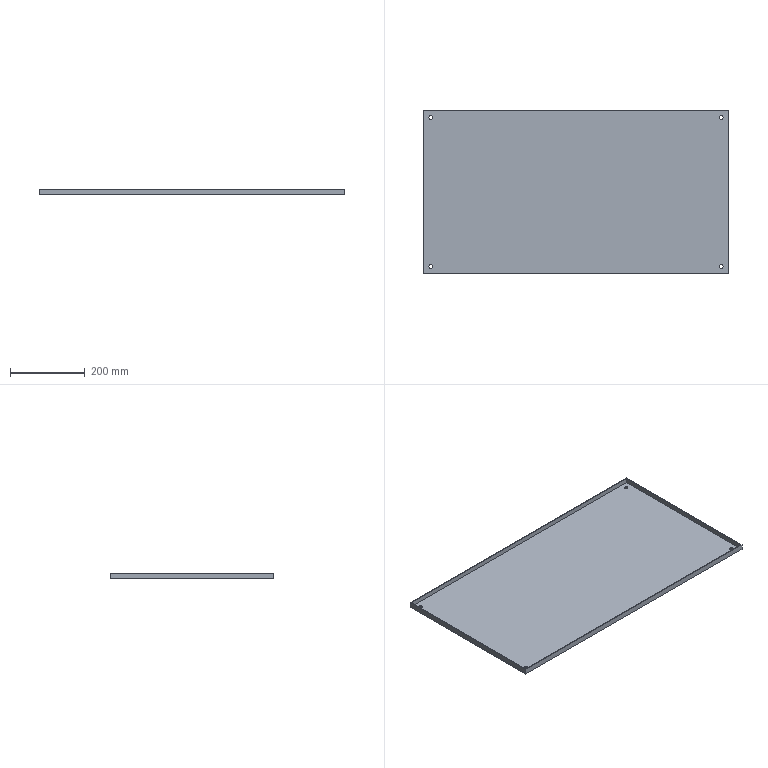Part | STEP file | 11-FGJJ-01111 | 1 solid | 19 faces | box 820 x 440 x 15 mm | volume 786284 mm3 | plane 11 | cylinder 8 | commonest cylinder face diameters 10 x8
STEP:
#1=CARTESIAN_POINT('',(-395.,200.,2.));
#2=VERTEX_POINT('',#1);
#3=CARTESIAN_POINT('',(-385.,200.,2.));
#4=VERTEX_POINT('',#3);
#5=CARTESIAN_POINT('',(-390.,200.,2.));
#6=DIRECTION('',(0.,0.,1.));
#7=DIRECTION('',(1.,0.,0.));
#8=AXIS2_PLACEMENT_3D('',#5,#6,#7);
#9=CIRCLE('',#8,5.);
#10=EDGE_CURVE('',#2,#4,#9,.T.);
#11=ORIENTED_EDGE('',*,*,#10,.T.);
#12=CARTESIAN_POINT('',(-385.,200.,0.));
#13=VERTEX_POINT('',#12);
#14=CARTESIAN_POINT('',(-385.,200.,44.));
#15=DIRECTION('',(0.,0.,-1.));
#16=VECTOR('',#15,1000.);
#17=LINE('',#14,#16);
#18=EDGE_CURVE('',#4,#13,#17,.T.);
#19=ORIENTED_EDGE('',*,*,#18,.T.);
#20=CARTESIAN_POINT('',(-395.,200.,0.));
#21=VERTEX_POINT('',#20);
#22=CARTESIAN_POINT('',(-390.,200.,0.));
#23=DIRECTION('',(0.,0.,-1.));
#24=DIRECTION('',(-1.,0.,0.));
#25=AXIS2_PLACEMENT_3D('',#22,#23,#24);
#26=CIRCLE('',#25,5.);
#27=EDGE_CURVE('',#13,#21,#26,.T.);
#28=ORIENTED_EDGE('',*,*,#27,.T.);
#29=CARTESIAN_POINT('',(-395.,200.,44.));
#30=DIRECTION('',(0.,0.,-1.));
#31=VECTOR('',#30,1000.);
#32=LINE('',#29,#31);
#33=EDGE_CURVE('',#2,#21,#32,.T.);
#34=ORIENTED_EDGE('',*,*,#33,.F.);
#35=EDGE_LOOP('',(#11,#19,#28,#34));
#36=FACE_OUTER_BOUND('',#35,.T.);
#37=CARTESIAN_POINT('',(-390.,200.,44.));
#38=DIRECTION('',(0.,0.,-1.));
#39=DIRECTION('',(-1.,0.,0.));
#40=AXIS2_PLACEMENT_3D('',#37,#38,#39);
#41=CYLINDRICAL_SURFACE('',#40,5.);
#42=ADVANCED_FACE('',(#36),#41,.F.);
#43=CARTESIAN_POINT('',(385.,-200.,2.));
#44=VERTEX_POINT('',#43);
#45=CARTESIAN_POINT('',(395.,-200.,2.));
#46=VERTEX_POINT('',#45);
#47=CARTESIAN_POINT('',(390.,-200.,2.));
#48=DIRECTION('',(0.,0.,1.));
#49=DIRECTION('',(1.,0.,0.));
#50=AXIS2_PLACEMENT_3D('',#47,#48,#49);
#51=CIRCLE('',#50,5.);
#52=EDGE_CURVE('',#44,#46,#51,.T.);
#53=ORIENTED_EDGE('',*,*,#52,.T.);
#54=CARTESIAN_POINT('',(395.,-200.,0.));
#55=VERTEX_POINT('',#54);
#56=CARTESIAN_POINT('',(395.,-200.,44.));
#57=DIRECTION('',(0.,0.,-1.));
#58=VECTOR('',#57,1000.);
#59=LINE('',#56,#58);
#60=EDGE_CURVE('',#46,#55,#59,.T.);
#61=ORIENTED_EDGE('',*,*,#60,.T.);
#62=CARTESIAN_POINT('',(385.,-200.,0.));
#63=VERTEX_POINT('',#62);
#64=CARTESIAN_POINT('',(390.,-200.,0.));
#65=DIRECTION('',(0.,0.,-1.));
#66=DIRECTION('',(-1.,0.,0.));
#67=AXIS2_PLACEMENT_3D('',#64,#65,#66);
#68=CIRCLE('',#67,5.);
#69=EDGE_CURVE('',#55,#63,#68,.T.);
#70=ORIENTED_EDGE('',*,*,#69,.T.);
#71=CARTESIAN_POINT('',(385.,-200.,44.));
#72=DIRECTION('',(0.,0.,-1.));
#73=VECTOR('',#72,1000.);
#74=LINE('',#71,#73);
#75=EDGE_CURVE('',#44,#63,#74,.T.);
#76=ORIENTED_EDGE('',*,*,#75,.F.);
#77=EDGE_LOOP('',(#53,#61,#70,#76));
#78=FACE_OUTER_BOUND('',#77,.T.);
#79=CARTESIAN_POINT('',(390.,-200.,44.));
#80=DIRECTION('',(0.,0.,-1.));
#81=DIRECTION('',(-1.,0.,0.));
#82=AXIS2_PLACEMENT_3D('',#79,#80,#81);
#83=CYLINDRICAL_SURFACE('',#82,5.);
#84=ADVANCED_FACE('',(#78),#83,.F.);
#85=CARTESIAN_POINT('',(-395.,-200.,2.));
#86=VERTEX_POINT('',#85);
#87=CARTESIAN_POINT('',(-385.,-200.,2.));
#88=VERTEX_POINT('',#87);
#89=CARTESIAN_POINT('',(-390.,-200.,2.));
#90=DIRECTION('',(0.,0.,1.));
#91=DIRECTION('',(1.,0.,0.));
#92=AXIS2_PLACEMENT_3D('',#89,#90,#91);
#93=CIRCLE('',#92,5.);
#94=EDGE_CURVE('',#86,#88,#93,.T.);
#95=ORIENTED_EDGE('',*,*,#94,.T.);
#96=CARTESIAN_POINT('',(-385.,-200.,0.));
#97=VERTEX_POINT('',#96);
#98=CARTESIAN_POINT('',(-385.,-200.,44.));
#99=DIRECTION('',(0.,0.,-1.));
#100=VECTOR('',#99,1000.);
#101=LINE('',#98,#100);
#102=EDGE_CURVE('',#88,#97,#101,.T.);
#103=ORIENTED_EDGE('',*,*,#102,.T.);
#104=CARTESIAN_POINT('',(-395.,-200.,0.));
#105=VERTEX_POINT('',#104);
#106=CARTESIAN_POINT('',(-390.,-200.,0.));
#107=DIRECTION('',(0.,0.,-1.));
#108=DIRECTION('',(-1.,0.,0.));
#109=AXIS2_PLACEMENT_3D('',#106,#107,#108);
#110=CIRCLE('',#109,5.);
#111=EDGE_CURVE('',#97,#105,#110,.T.);
#112=ORIENTED_EDGE('',*,*,#111,.T.);
#113=CARTESIAN_POINT('',(-395.,-200.,44.));
#114=DIRECTION('',(0.,0.,-1.));
#115=VECTOR('',#114,1000.);
#116=LINE('',#113,#115);
#117=EDGE_CURVE('',#86,#105,#116,.T.);
#118=ORIENTED_EDGE('',*,*,#117,.F.);
#119=EDGE_LOOP('',(#95,#103,#112,#118));
#120=FACE_OUTER_BOUND('',#119,.T.);
#121=CARTESIAN_POINT('',(-390.,-200.,44.));
#122=DIRECTION('',(0.,0.,-1.));
#123=DIRECTION('',(-1.,0.,0.));
#124=AXIS2_PLACEMENT_3D('',#121,#122,#123);
#125=CYLINDRICAL_SURFACE('',#124,5.);
#126=ADVANCED_FACE('',(#120),#125,.F.);
#127=CARTESIAN_POINT('',(385.,200.,2.));
#128=VERTEX_POINT('',#127);
#129=CARTESIAN_POINT('',(395.,200.,2.));
#130=VERTEX_POINT('',#129);
#131=CARTESIAN_POINT('',(390.,200.,2.));
#132=DIRECTION('',(0.,0.,1.));
#133=DIRECTION('',(1.,0.,0.));
#134=AXIS2_PLACEMENT_3D('',#131,#132,#133);
#135=CIRCLE('',#134,5.);
#136=EDGE_CURVE('',#128,#130,#135,.T.);
#137=ORIENTED_EDGE('',*,*,#136,.T.);
#138=CARTESIAN_POINT('',(395.,200.,0.));
#139=VERTEX_POINT('',#138);
#140=CARTESIAN_POINT('',(395.,200.,44.));
#141=DIRECTION('',(0.,0.,-1.));
#142=VECTOR('',#141,1000.);
#143=LINE('',#140,#142);
#144=EDGE_CURVE('',#130,#139,#143,.T.);
#145=ORIENTED_EDGE('',*,*,#144,.T.);
#146=CARTESIAN_POINT('',(385.,200.,0.));
#147=VERTEX_POINT('',#146);
#148=CARTESIAN_POINT('',(390.,200.,0.));
#149=DIRECTION('',(0.,0.,-1.));
#150=DIRECTION('',(-1.,0.,0.));
#151=AXIS2_PLACEMENT_3D('',#148,#149,#150);
#152=CIRCLE('',#151,5.);
#153=EDGE_CURVE('',#139,#147,#152,.T.);
#154=ORIENTED_EDGE('',*,*,#153,.T.);
#155=CARTESIAN_POINT('',(385.,200.,44.));
#156=DIRECTION('',(0.,0.,-1.));
#157=VECTOR('',#156,1000.);
#158=LINE('',#155,#157);
#159=EDGE_CURVE('',#128,#147,#158,.T.);
#160=ORIENTED_EDGE('',*,*,#159,.F.);
#161=EDGE_LOOP('',(#137,#145,#154,#160));
#162=FACE_OUTER_BOUND('',#161,.T.);
#163=CARTESIAN_POINT('',(390.,200.,44.));
#164=DIRECTION('',(0.,0.,-1.));
#165=DIRECTION('',(-1.,0.,0.));
#166=AXIS2_PLACEMENT_3D('',#163,#164,#165);
#167=CYLINDRICAL_SURFACE('',#166,5.);
#168=ADVANCED_FACE('',(#162),#167,.F.);
#169=CARTESIAN_POINT('',(410.,-220.,0.));
#170=VERTEX_POINT('',#169);
#171=CARTESIAN_POINT('',(410.,220.,0.));
#172=VERTEX_POINT('',#171);
#173=CARTESIAN_POINT('',(410.,220.,0.));
#174=DIRECTION('',(0.,1.,0.));
#175=VECTOR('',#174,1000.);
#176=LINE('',#173,#175);
#177=EDGE_CURVE('',#170,#172,#176,.T.);
#178=ORIENTED_EDGE('',*,*,#177,.T.);
#179=CARTESIAN_POINT('',(410.,220.,15.));
#180=VERTEX_POINT('',#179);
#181=CARTESIAN_POINT('',(410.,220.,15.));
#182=DIRECTION('',(0.,0.,-1.));
#183=VECTOR('',#182,1000.);
#184=LINE('',#181,#183);
#185=EDGE_CURVE('',#180,#172,#184,.T.);
#186=ORIENTED_EDGE('',*,*,#185,.F.);
#187=CARTESIAN_POINT('',(410.,-220.,15.));
#188=VERTEX_POINT('',#187);
#189=CARTESIAN_POINT('',(410.,220.,15.));
#190=DIRECTION('',(0.,1.,0.));
#191=VECTOR('',#190,1000.);
#192=LINE('',#189,#191);
#193=EDGE_CURVE('',#188,#180,#192,.T.);
#194=ORIENTED_EDGE('',*,*,#193,.F.);
#195=CARTESIAN_POINT('',(410.,-220.,15.));
#196=DIRECTION('',(0.,0.,-1.));
#197=VECTOR('',#196,1000.);
#198=LINE('',#195,#197);
#199=EDGE_CURVE('',#188,#170,#198,.T.);
#200=ORIENTED_EDGE('',*,*,#199,.T.);
#201=EDGE_LOOP('',(#178,#186,#194,#200));
#202=FACE_OUTER_BOUND('',#201,.T.);
#203=CARTESIAN_POINT('',(410.,220.,15.));
#204=DIRECTION('',(-1.,0.,0.));
#205=DIRECTION('',(0.,-1.,0.));
#206=AXIS2_PLACEMENT_3D('',#203,#204,#205);
#207=PLANE('',#206);
#208=ADVANCED_FACE('',(#202),#207,.F.);
#209=CARTESIAN_POINT('',(-410.,220.,0.));
#210=VERTEX_POINT('',#209);
#211=CARTESIAN_POINT('',(-410.,220.,0.));
#212=DIRECTION('',(-1.,0.,0.));
#213=VECTOR('',#212,1000.);
#214=LINE('',#211,#213);
#215=EDGE_CURVE('',#172,#210,#214,.T.);
#216=ORIENTED_EDGE('',*,*,#215,.T.);
#217=CARTESIAN_POINT('',(-410.,220.,15.));
#218=VERTEX_POINT('',#217);
#219=CARTESIAN_POINT('',(-410.,220.,15.));
#220=DIRECTION('',(0.,0.,-1.));
#221=VECTOR('',#220,1000.);
#222=LINE('',#219,#221);
#223=EDGE_CURVE('',#218,#210,#222,.T.);
#224=ORIENTED_EDGE('',*,*,#223,.F.);
#225=CARTESIAN_POINT('',(-410.,220.,15.));
#226=DIRECTION('',(-1.,0.,0.));
#227=VECTOR('',#226,1000.);
#228=LINE('',#225,#227);
#229=EDGE_CURVE('',#180,#218,#228,.T.);
#230=ORIENTED_EDGE('',*,*,#229,.F.);
#231=ORIENTED_EDGE('',*,*,#185,.T.);
#232=EDGE_LOOP('',(#216,#224,#230,#231));
#233=FACE_OUTER_BOUND('',#232,.T.);
#234=CARTESIAN_POINT('',(-410.,220.,15.));
#235=DIRECTION('',(0.,-1.,0.));
#236=DIRECTION('',(0.,0.,-1.));
#237=AXIS2_PLACEMENT_3D('',#234,#235,#236);
#238=PLANE('',#237);
#239=ADVANCED_FACE('',(#233),#238,.F.);
#240=CARTESIAN_POINT('',(-410.,-220.,0.));
#241=VERTEX_POINT('',#240);
#242=CARTESIAN_POINT('',(-410.,220.,0.));
#243=DIRECTION('',(0.,-1.,0.));
#244=VECTOR('',#243,1000.);
#245=LINE('',#242,#244);
#246=EDGE_CURVE('',#210,#241,#245,.T.);
#247=ORIENTED_EDGE('',*,*,#246,.T.);
#248=CARTESIAN_POINT('',(-410.,-220.,15.));
#249=VERTEX_POINT('',#248);
#250=CARTESIAN_POINT('',(-410.,-220.,15.));
#251=DIRECTION('',(0.,0.,-1.));
#252=VECTOR('',#251,1000.);
#253=LINE('',#250,#252);
#254=EDGE_CURVE('',#249,#241,#253,.T.);
#255=ORIENTED_EDGE('',*,*,#254,.F.);
#256=CARTESIAN_POINT('',(-410.,220.,15.));
#257=DIRECTION('',(0.,-1.,0.));
#258=VECTOR('',#257,1000.);
#259=LINE('',#256,#258);
#260=EDGE_CURVE('',#218,#249,#259,.T.);
#261=ORIENTED_EDGE('',*,*,#260,.F.);
#262=ORIENTED_EDGE('',*,*,#223,.T.);
#263=EDGE_LOOP('',(#247,#255,#261,#262));
#264=FACE_OUTER_BOUND('',#263,.T.);
#265=CARTESIAN_POINT('',(-410.,220.,15.));
#266=DIRECTION('',(1.,0.,0.));
#267=DIRECTION('',(0.,1.,0.));
#268=AXIS2_PLACEMENT_3D('',#265,#266,#267);
#269=PLANE('',#268);
#270=ADVANCED_FACE('',(#264),#269,.F.);
#271=CARTESIAN_POINT('',(-410.,-220.,0.));
#272=DIRECTION('',(1.,0.,0.));
#273=VECTOR('',#272,1000.);
#274=LINE('',#271,#273);
#275=EDGE_CURVE('',#241,#170,#274,.T.);
#276=ORIENTED_EDGE('',*,*,#275,.T.);
#277=ORIENTED_EDGE('',*,*,#199,.F.);
#278=CARTESIAN_POINT('',(-410.,-220.,15.));
#279=DIRECTION('',(1.,0.,0.));
#280=VECTOR('',#279,1000.);
#281=LINE('',#278,#280);
#282=EDGE_CURVE('',#249,#188,#281,.T.);
#283=ORIENTED_EDGE('',*,*,#282,.F.);
#284=ORIENTED_EDGE('',*,*,#254,.T.);
#285=EDGE_LOOP('',(#276,#277,#283,#284));
#286=FACE_OUTER_BOUND('',#285,.T.);
#287=CARTESIAN_POINT('',(-410.,-220.,15.));
#288=DIRECTION('',(0.,1.,0.));
#289=DIRECTION('',(0.,0.,1.));
#290=AXIS2_PLACEMENT_3D('',#287,#288,#289);
#291=PLANE('',#290);
#292=ADVANCED_FACE('',(#286),#291,.F.);
#293=CARTESIAN_POINT('',(408.,-218.,15.));
#294=VERTEX_POINT('',#293);
#295=CARTESIAN_POINT('',(408.,218.,15.));
#296=VERTEX_POINT('',#295);
#297=CARTESIAN_POINT('',(408.,220.,15.));
#298=DIRECTION('',(0.,1.,0.));
#299=VECTOR('',#298,1000.);
#300=LINE('',#297,#299);
#301=EDGE_CURVE('',#294,#296,#300,.T.);
#302=ORIENTED_EDGE('',*,*,#301,.F.);
#303=CARTESIAN_POINT('',(-408.,-218.,15.));
#304=VERTEX_POINT('',#303);
#305=CARTESIAN_POINT('',(-410.,-218.,15.));
#306=DIRECTION('',(1.,0.,0.));
#307=VECTOR('',#306,1000.);
#308=LINE('',#305,#307);
#309=EDGE_CURVE('',#304,#294,#308,.T.);
#310=ORIENTED_EDGE('',*,*,#309,.F.);
#311=CARTESIAN_POINT('',(-408.,218.,15.));
#312=VERTEX_POINT('',#311);
#313=CARTESIAN_POINT('',(-408.,220.,15.));
#314=DIRECTION('',(0.,-1.,0.));
#315=VECTOR('',#314,1000.);
#316=LINE('',#313,#315);
#317=EDGE_CURVE('',#312,#304,#316,.T.);
#318=ORIENTED_EDGE('',*,*,#317,.F.);
#319=CARTESIAN_POINT('',(-410.,218.,15.));
#320=DIRECTION('',(-1.,0.,0.));
#321=VECTOR('',#320,1000.);
#322=LINE('',#319,#321);
#323=EDGE_CURVE('',#296,#312,#322,.T.);
#324=ORIENTED_EDGE('',*,*,#323,.F.);
#325=EDGE_LOOP('',(#302,#310,#318,#324));
#326=FACE_BOUND('',#325,.T.);
#327=ORIENTED_EDGE('',*,*,#193,.T.);
#328=ORIENTED_EDGE('',*,*,#229,.T.);
#329=ORIENTED_EDGE('',*,*,#260,.T.);
#330=ORIENTED_EDGE('',*,*,#282,.T.);
#331=EDGE_LOOP('',(#327,#328,#329,#330));
#332=FACE_OUTER_BOUND('',#331,.T.);
#333=CARTESIAN_POINT('',(0.,0.,15.));
#334=DIRECTION('',(0.,0.,1.));
#335=DIRECTION('',(1.,0.,0.));
#336=AXIS2_PLACEMENT_3D('',#333,#334,#335);
#337=PLANE('',#336);
#338=ADVANCED_FACE('',(#326,#332),#337,.T.);
#339=CARTESIAN_POINT('',(-390.,200.,0.));
#340=DIRECTION('',(0.,0.,-1.));
#341=DIRECTION('',(-1.,0.,0.));
#342=AXIS2_PLACEMENT_3D('',#339,#340,#341);
#343=CIRCLE('',#342,5.);
#344=EDGE_CURVE('',#21,#13,#343,.T.);
#345=ORIENTED_EDGE('',*,*,#344,.F.);
#346=ORIENTED_EDGE('',*,*,#27,.F.);
#347=EDGE_LOOP('',(#345,#346));
#348=FACE_BOUND('',#347,.T.);
#349=CARTESIAN_POINT('',(390.,-200.,0.));
#350=DIRECTION('',(0.,0.,-1.));
#351=DIRECTION('',(-1.,0.,0.));
#352=AXIS2_PLACEMENT_3D('',#349,#350,#351);
#353=CIRCLE('',#352,5.);
#354=EDGE_CURVE('',#63,#55,#353,.T.);
#355=ORIENTED_EDGE('',*,*,#354,.F.);
#356=ORIENTED_EDGE('',*,*,#69,.F.);
#357=EDGE_LOOP('',(#355,#356));
#358=FACE_BOUND('',#357,.T.);
#359=CARTESIAN_POINT('',(-390.,-200.,0.));
#360=DIRECTION('',(0.,0.,-1.));
#361=DIRECTION('',(-1.,0.,0.));
#362=AXIS2_PLACEMENT_3D('',#359,#360,#361);
#363=CIRCLE('',#362,5.);
#364=EDGE_CURVE('',#105,#97,#363,.T.);
#365=ORIENTED_EDGE('',*,*,#364,.F.);
#366=ORIENTED_EDGE('',*,*,#111,.F.);
#367=EDGE_LOOP('',(#365,#366));
#368=FACE_BOUND('',#367,.T.);
#369=CARTESIAN_POINT('',(390.,200.,0.));
#370=DIRECTION('',(0.,0.,-1.));
#371=DIRECTION('',(-1.,0.,0.));
#372=AXIS2_PLACEMENT_3D('',#369,#370,#371);
#373=CIRCLE('',#372,5.);
#374=EDGE_CURVE('',#147,#139,#373,.T.);
#375=ORIENTED_EDGE('',*,*,#374,.F.);
#376=ORIENTED_EDGE('',*,*,#153,.F.);
#377=EDGE_LOOP('',(#375,#376));
#378=FACE_BOUND('',#377,.T.);
#379=ORIENTED_EDGE('',*,*,#177,.F.);
#380=ORIENTED_EDGE('',*,*,#275,.F.);
#381=ORIENTED_EDGE('',*,*,#246,.F.);
#382=ORIENTED_EDGE('',*,*,#215,.F.);
#383=EDGE_LOOP('',(#379,#380,#381,#382));
#384=FACE_OUTER_BOUND('',#383,.T.);
#385=CARTESIAN_POINT('',(0.,0.,0.));
#386=DIRECTION('',(0.,0.,1.));
#387=DIRECTION('',(1.,0.,0.));
#388=AXIS2_PLACEMENT_3D('',#385,#386,#387);
#389=PLANE('',#388);
#390=ADVANCED_FACE('',(#348,#358,#368,#378,#384),#389,.F.);
#391=CARTESIAN_POINT('',(408.,-218.,2.));
#392=VERTEX_POINT('',#391);
#393=CARTESIAN_POINT('',(408.,218.,2.));
#394=VERTEX_POINT('',#393);
#395=CARTESIAN_POINT('',(408.,220.,2.));
#396=DIRECTION('',(0.,1.,0.));
#397=VECTOR('',#396,1000.);
#398=LINE('',#395,#397);
#399=EDGE_CURVE('',#392,#394,#398,.T.);
#400=ORIENTED_EDGE('',*,*,#399,.F.);
#401=CARTESIAN_POINT('',(408.,-218.,15.));
#402=DIRECTION('',(0.,0.,-1.));
#403=VECTOR('',#402,1000.);
#404=LINE('',#401,#403);
#405=EDGE_CURVE('',#294,#392,#404,.T.);
#406=ORIENTED_EDGE('',*,*,#405,.F.);
#407=ORIENTED_EDGE('',*,*,#301,.T.);
#408=CARTESIAN_POINT('',(408.,218.,15.));
#409=DIRECTION('',(0.,0.,-1.));
#410=VECTOR('',#409,1000.);
#411=LINE('',#408,#410);
#412=EDGE_CURVE('',#296,#394,#411,.T.);
#413=ORIENTED_EDGE('',*,*,#412,.T.);
#414=EDGE_LOOP('',(#400,#406,#407,#413));
#415=FACE_OUTER_BOUND('',#414,.T.);
#416=CARTESIAN_POINT('',(408.,220.,15.));
#417=DIRECTION('',(-1.,0.,0.));
#418=DIRECTION('',(0.,-1.,0.));
#419=AXIS2_PLACEMENT_3D('',#416,#417,#418);
#420=PLANE('',#419);
#421=ADVANCED_FACE('',(#415),#420,.T.);
#422=CARTESIAN_POINT('',(-408.,218.,2.));
#423=VERTEX_POINT('',#422);
#424=CARTESIAN_POINT('',(-410.,218.,2.));
#425=DIRECTION('',(-1.,0.,0.));
#426=VECTOR('',#425,1000.);
#427=LINE('',#424,#426);
#428=EDGE_CURVE('',#394,#423,#427,.T.);
#429=ORIENTED_EDGE('',*,*,#428,.F.);
#430=ORIENTED_EDGE('',*,*,#412,.F.);
#431=ORIENTED_EDGE('',*,*,#323,.T.);
#432=CARTESIAN_POINT('',(-408.,218.,15.));
#433=DIRECTION('',(0.,0.,-1.));
#434=VECTOR('',#433,1000.);
#435=LINE('',#432,#434);
#436=EDGE_CURVE('',#312,#423,#435,.T.);
#437=ORIENTED_EDGE('',*,*,#436,.T.);
#438=EDGE_LOOP('',(#429,#430,#431,#437));
#439=FACE_OUTER_BOUND('',#438,.T.);
#440=CARTESIAN_POINT('',(-410.,218.,15.));
#441=DIRECTION('',(0.,-1.,0.));
#442=DIRECTION('',(0.,0.,-1.));
#443=AXIS2_PLACEMENT_3D('',#440,#441,#442);
#444=PLANE('',#443);
#445=ADVANCED_FACE('',(#439),#444,.T.);
#446=CARTESIAN_POINT('',(-408.,-218.,2.));
#447=VERTEX_POINT('',#446);
#448=CARTESIAN_POINT('',(-408.,220.,2.));
#449=DIRECTION('',(0.,-1.,0.));
#450=VECTOR('',#449,1000.);
#451=LINE('',#448,#450);
#452=EDGE_CURVE('',#423,#447,#451,.T.);
#453=ORIENTED_EDGE('',*,*,#452,.F.);
#454=ORIENTED_EDGE('',*,*,#436,.F.);
#455=ORIENTED_EDGE('',*,*,#317,.T.);
#456=CARTESIAN_POINT('',(-408.,-218.,15.));
#457=DIRECTION('',(0.,0.,-1.));
#458=VECTOR('',#457,1000.);
#459=LINE('',#456,#458);
#460=EDGE_CURVE('',#304,#447,#459,.T.);
#461=ORIENTED_EDGE('',*,*,#460,.T.);
#462=EDGE_LOOP('',(#453,#454,#455,#461));
#463=FACE_OUTER_BOUND('',#462,.T.);
#464=CARTESIAN_POINT('',(-408.,220.,15.));
#465=DIRECTION('',(1.,0.,0.));
#466=DIRECTION('',(0.,1.,0.));
#467=AXIS2_PLACEMENT_3D('',#464,#465,#466);
#468=PLANE('',#467);
#469=ADVANCED_FACE('',(#463),#468,.T.);
#470=CARTESIAN_POINT('',(-410.,-218.,2.));
#471=DIRECTION('',(1.,0.,0.));
#472=VECTOR('',#471,1000.);
#473=LINE('',#470,#472);
#474=EDGE_CURVE('',#447,#392,#473,.T.);
#475=ORIENTED_EDGE('',*,*,#474,.F.);
#476=ORIENTED_EDGE('',*,*,#460,.F.);
#477=ORIENTED_EDGE('',*,*,#309,.T.);
#478=ORIENTED_EDGE('',*,*,#405,.T.);
#479=EDGE_LOOP('',(#475,#476,#477,#478));
#480=FACE_OUTER_BOUND('',#479,.T.);
#481=CARTESIAN_POINT('',(-410.,-218.,15.));
#482=DIRECTION('',(0.,1.,0.));
#483=DIRECTION('',(0.,0.,1.));
#484=AXIS2_PLACEMENT_3D('',#481,#482,#483);
#485=PLANE('',#484);
#486=ADVANCED_FACE('',(#480),#485,.T.);
#487=ORIENTED_EDGE('',*,*,#10,.F.);
#488=CARTESIAN_POINT('',(-390.,200.,2.));
#489=DIRECTION('',(0.,0.,1.));
#490=DIRECTION('',(1.,0.,0.));
#491=AXIS2_PLACEMENT_3D('',#488,#489,#490);
#492=CIRCLE('',#491,5.);
#493=EDGE_CURVE('',#4,#2,#492,.T.);
#494=ORIENTED_EDGE('',*,*,#493,.F.);
#495=EDGE_LOOP('',(#487,#494));
#496=FACE_BOUND('',#495,.T.);
#497=ORIENTED_EDGE('',*,*,#52,.F.);
#498=CARTESIAN_POINT('',(390.,-200.,2.));
#499=DIRECTION('',(0.,0.,1.));
#500=DIRECTION('',(1.,0.,0.));
#501=AXIS2_PLACEMENT_3D('',#498,#499,#500);
#502=CIRCLE('',#501,5.);
#503=EDGE_CURVE('',#46,#44,#502,.T.);
#504=ORIENTED_EDGE('',*,*,#503,.F.);
#505=EDGE_LOOP('',(#497,#504));
#506=FACE_BOUND('',#505,.T.);
#507=ORIENTED_EDGE('',*,*,#94,.F.);
#508=CARTESIAN_POINT('',(-390.,-200.,2.));
#509=DIRECTION('',(0.,0.,1.));
#510=DIRECTION('',(1.,0.,0.));
#511=AXIS2_PLACEMENT_3D('',#508,#509,#510);
#512=CIRCLE('',#511,5.);
#513=EDGE_CURVE('',#88,#86,#512,.T.);
#514=ORIENTED_EDGE('',*,*,#513,.F.);
#515=EDGE_LOOP('',(#507,#514));
#516=FACE_BOUND('',#515,.T.);
#517=ORIENTED_EDGE('',*,*,#136,.F.);
#518=CARTESIAN_POINT('',(390.,200.,2.));
#519=DIRECTION('',(0.,0.,1.));
#520=DIRECTION('',(1.,0.,0.));
#521=AXIS2_PLACEMENT_3D('',#518,#519,#520);
#522=CIRCLE('',#521,5.);
#523=EDGE_CURVE('',#130,#128,#522,.T.);
#524=ORIENTED_EDGE('',*,*,#523,.F.);
#525=EDGE_LOOP('',(#517,#524));
#526=FACE_BOUND('',#525,.T.);
#527=ORIENTED_EDGE('',*,*,#399,.T.);
#528=ORIENTED_EDGE('',*,*,#428,.T.);
#529=ORIENTED_EDGE('',*,*,#452,.T.);
#530=ORIENTED_EDGE('',*,*,#474,.T.);
#531=EDGE_LOOP('',(#527,#528,#529,#530));
#532=FACE_OUTER_BOUND('',#531,.T.);
#533=CARTESIAN_POINT('',(0.,0.,2.));
#534=DIRECTION('',(0.,0.,1.));
#535=DIRECTION('',(1.,0.,0.));
#536=AXIS2_PLACEMENT_3D('',#533,#534,#535);
#537=PLANE('',#536);
#538=ADVANCED_FACE('',(#496,#506,#516,#526,#532),#537,.T.);
#539=ORIENTED_EDGE('',*,*,#144,.F.);
#540=ORIENTED_EDGE('',*,*,#523,.T.);
#541=ORIENTED_EDGE('',*,*,#159,.T.);
#542=ORIENTED_EDGE('',*,*,#374,.T.);
#543=EDGE_LOOP('',(#539,#540,#541,#542));
#544=FACE_OUTER_BOUND('',#543,.T.);
#545=CARTESIAN_POINT('',(390.,200.,44.));
#546=DIRECTION('',(0.,0.,-1.));
#547=DIRECTION('',(-1.,0.,0.));
#548=AXIS2_PLACEMENT_3D('',#545,#546,#547);
#549=CYLINDRICAL_SURFACE('',#548,5.);
#550=ADVANCED_FACE('',(#544),#549,.F.);
#551=ORIENTED_EDGE('',*,*,#102,.F.);
#552=ORIENTED_EDGE('',*,*,#513,.T.);
#553=ORIENTED_EDGE('',*,*,#117,.T.);
#554=ORIENTED_EDGE('',*,*,#364,.T.);
#555=EDGE_LOOP('',(#551,#552,#553,#554));
#556=FACE_OUTER_BOUND('',#555,.T.);
#557=CARTESIAN_POINT('',(-390.,-200.,44.));
#558=DIRECTION('',(0.,0.,-1.));
#559=DIRECTION('',(-1.,0.,0.));
#560=AXIS2_PLACEMENT_3D('',#557,#558,#559);
#561=CYLINDRICAL_SURFACE('',#560,5.);
#562=ADVANCED_FACE('',(#556),#561,.F.);
#563=ORIENTED_EDGE('',*,*,#60,.F.);
#564=ORIENTED_EDGE('',*,*,#503,.T.);
#565=ORIENTED_EDGE('',*,*,#75,.T.);
#566=ORIENTED_EDGE('',*,*,#354,.T.);
#567=EDGE_LOOP('',(#563,#564,#565,#566));
#568=FACE_OUTER_BOUND('',#567,.T.);
#569=CARTESIAN_POINT('',(390.,-200.,44.));
#570=DIRECTION('',(0.,0.,-1.));
#571=DIRECTION('',(-1.,0.,0.));
#572=AXIS2_PLACEMENT_3D('',#569,#570,#571);
#573=CYLINDRICAL_SURFACE('',#572,5.);
#574=ADVANCED_FACE('',(#568),#573,.F.);
#575=ORIENTED_EDGE('',*,*,#18,.F.);
#576=ORIENTED_EDGE('',*,*,#493,.T.);
#577=ORIENTED_EDGE('',*,*,#33,.T.);
#578=ORIENTED_EDGE('',*,*,#344,.T.);
#579=EDGE_LOOP('',(#575,#576,#577,#578));
#580=FACE_OUTER_BOUND('',#579,.T.);
#581=CARTESIAN_POINT('',(-390.,200.,44.));
#582=DIRECTION('',(0.,0.,-1.));
#583=DIRECTION('',(-1.,0.,0.));
#584=AXIS2_PLACEMENT_3D('',#581,#582,#583);
#585=CYLINDRICAL_SURFACE('',#584,5.);
#586=ADVANCED_FACE('',(#580),#585,.F.);
#587=CLOSED_SHELL('',(#42,#84,#126,#168,#208,#239,#270,#292,#338,#390,#421,#445,#469,#486,#538,#550,#562,#574,#586));
#588=MANIFOLD_SOLID_BREP('',#587);
#589=CARTESIAN_POINT('',(0.,0.,0.));
#590=DIRECTION('',(0.,0.,1.));
#591=DIRECTION('',(1.,0.,0.));
#592=AXIS2_PLACEMENT_3D('',#589,#590,#591);
#593=(LENGTH_UNIT()NAMED_UNIT(*)SI_UNIT(.MILLI.,.METRE.));
#594=UNCERTAINTY_MEASURE_WITH_UNIT(LENGTH_MEASURE(0.00001),#593,'','');
#595=(NAMED_UNIT(*)PLANE_ANGLE_UNIT()SI_UNIT($,.RADIAN.));
#596=(NAMED_UNIT(*)SI_UNIT($,.STERADIAN.)SOLID_ANGLE_UNIT());
#597=(GEOMETRIC_REPRESENTATION_CONTEXT(3)GLOBAL_UNCERTAINTY_ASSIGNED_CONTEXT((#594))GLOBAL_UNIT_ASSIGNED_CONTEXT((#593,#595,#596))REPRESENTATION_CONTEXT('',''));
#598=ADVANCED_BREP_SHAPE_REPRESENTATION('',(#588,#592),#597);